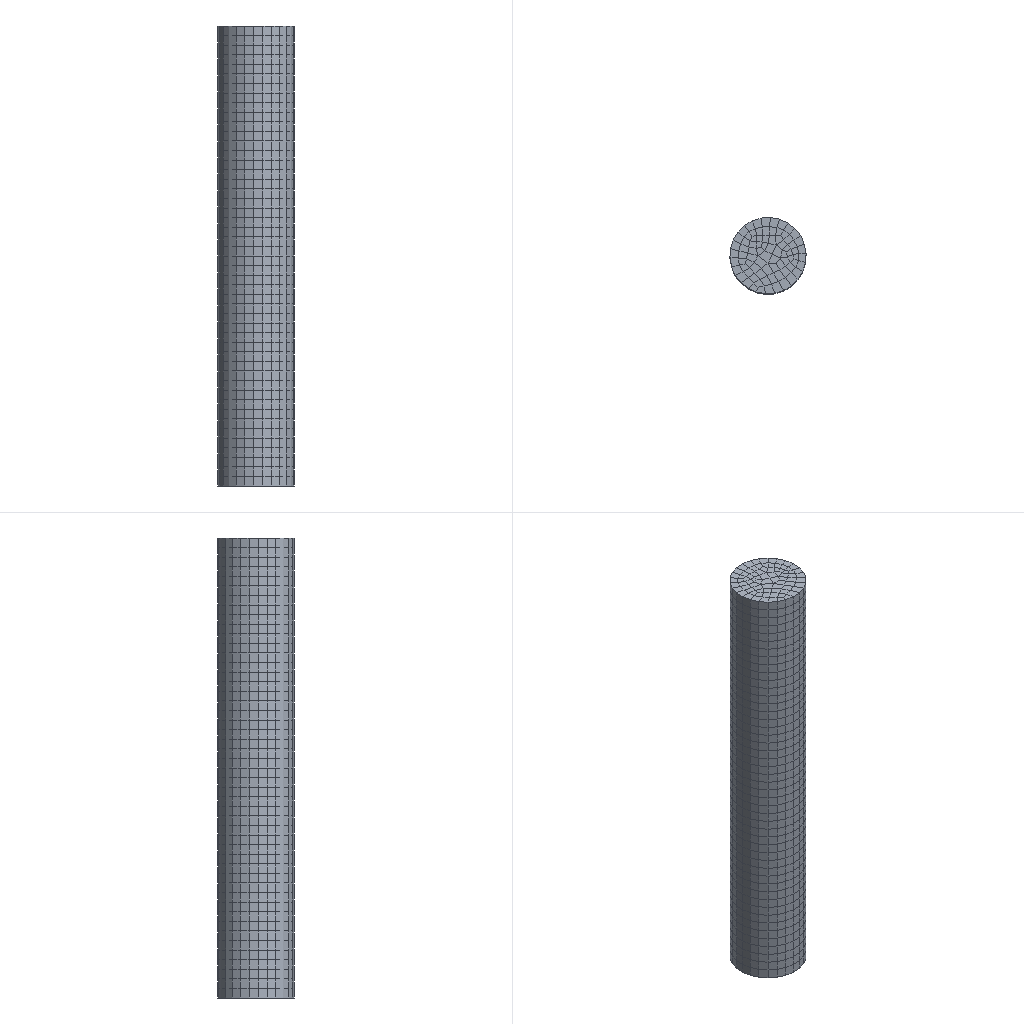Simulation study | abaqus
Set-up summary:
category,name,step,type,value,unit,region
solver,abaqus
solver,version,,,Abaqus/Explicit 2020
units,not stated in the deck,,not stated
analysis,deck,,transient,transient
load_step,Step-1,Step-1,transient
load_step,requested,,,1
mesh,nodes,,,17545
mesh,elements,,,16909
element_type,R3D3,,rigid,125
element_type,R3D4,,rigid,12992
element_type,C3D8R,,solid,3792
load,load commands in deck,,count,1
bc,support commands in deck,,count,7
material,TI,,in results
check,setup vs results,,match,"per instance, exact: element labels, types and connectivity; labels of the nodes the elements use; coordinates of those nodes at SINGLE_PRECISION in 3 of 3 instance(s)"
Abaqus input file, long lists of numbers shortened:
*Heading
** Job name: Job-1 Model name: Model-1
** Generated by: Abaqus/CAE 2020
*Preprint, echo=NO, model=NO, history=NO, contact=NO
**
** PARTS
**
*Part, name=chudun-2
*Node
      1,  -88.649,  -41.876,          90.
      2,  -88.649,  -41.876,         120.
** (8718 more lines like these left out)
*Element, type=R3D4
  1,    1,    7,  341,  388
  2,    7,    8,  342,  341
** (8690 more lines like these left out)
*Element, type=R3D3
6564, 7699, 6751, 7323
6565, 7752, 7314, 7227
** (54 more lines like these left out)
*Node
   8721,  -88.649,  -53.376,         120.
*Nset, nset=chudun-2-RefPt_, internal
8721,
*Elset, elset=chudun-2, generate
    1,  8748,     1
*End Part
**
*Part, name=chudun-4
*Node
      1,  -111.619,  -53.376,          15.
      2,  -111.619,  -53.376,          16.
** (4264 more lines like these left out)
*Element, type=R3D4
  1,   1,   6, 104,   2
  2,   6,   7, 105, 104
** (4298 more lines like these left out)
*Element, type=R3D3
1030, 1237, 1243, 1314
1031, 1266, 1262, 1236
** (67 more lines like these left out)
*Node
   4267,  -88.649,  -53.376,          15.
*Nset, nset=chudun-4-RefPt_, internal
4267,
*Elset, elset=chudun-4, generate
    1,  4369,     1
*End Part
**
*Part, name=xiancai
*Node
      1,   1.19,   3.819,   48.2
      2,  0.2415,   3.993,   48.2
** (4555 more lines like these left out)
*Element, type=C3D8R
   1,  109,   94,  133,  120,   16,    1,   40,   27
   2,  121,   95,  110,  134,   28,    2,   17,   41
** (3790 more lines like these left out)
*Nset, nset=Set-1, generate
    1,  4557,     1
*Elset, elset=Set-1, generate
    1,  3792,     1
** Section: Section-1
*Solid Section, elset=Set-1, material=ti
,
*End Part
**
**
** ASSEMBLY
**
*Assembly, name=Assembly
**
*Instance, name=xiancai-1, part=xiancai
          0.,           0.,        -104.
*End Instance
**
*Instance, name=chudun-2-1, part=chudun-2
   88.649,    53.376,        -120.
*End Instance
**
*Instance, name=chudun-4-1, part=chudun-4
   88.649,    53.376,        -120.
*End Instance
**
*Nset, nset=Set-2, instance=xiancai-1, generate
 4465,  4557,     1
*Elset, elset=Set-2, instance=xiancai-1, generate
 3714,  3792,     1
*Nset, nset=Set-3, instance=chudun-2-1
 8721,
*Nset, nset=Set-3, instance=chudun-4-1
 4267,
*Nset, nset=Set-4, instance=xiancai-1, generate
  1,  93,   1
*Elset, elset=Set-4, instance=xiancai-1, generate
  1,  79,   1
*Rigid Body, ref node=chudun-2-1.chudun-2-RefPt_, elset=chudun-2-1.chudun-2
*Rigid Body, ref node=chudun-4-1.chudun-4-RefPt_, elset=chudun-4-1.chudun-4
*End Assembly
*Amplitude, name=Amp-1
             0.,              0.,             0.1,              1.
**
** MATERIALS
**
*Material, name=ti
*Density
 3.5e-09,
*Elastic
45000., 0.28
*Plastic
300.,0.
**
** INTERACTION PROPERTIES
**
*Surface Interaction, name=IntProp-1
*Friction
 0.01,
*Surface Behavior, pressure-overclosure=HARD
** ----------------------------------------------------------------
**
** STEP: Step-1
**
*Step, name=Step-1, nlgeom=YES
*Dynamic, Explicit
, 0.1
*Bulk Viscosity
0.06, 1.2
** Mass Scaling: Semi-Automatic
**               Whole Model
*Fixed Mass Scaling, factor=5000.
**
** BOUNDARY CONDITIONS
**
** Name: BC-1 Type: 对称/反对称/完全固定
*Boundary
Set-3, ENCASTRE
** Name: BC-2 Type: 位移/转角
*Boundary, amplitude=Amp-1
Set-4, 1, 1
Set-4, 2, 2
Set-4, 3, 3, -25.
Set-4, 4, 4
Set-4, 5, 5
Set-4, 6, 6
**
** INTERACTIONS
**
** Interaction: Int-1
*Contact, op=NEW
*Contact Inclusions, ALL EXTERIOR
*Contact Property Assignment
 ,  , IntProp-1
**
** OUTPUT REQUESTS
**
*Restart, write, number interval=1, time marks=NO
**
** FIELD OUTPUT: F-Output-1
**
*Output, field, number interval=50
*Node Output
A, RF, RM, RT, U, V
*Element Output, directions=YES
E, EVF, LE, MISES, PE, PEEQ, PEEQVAVG, PEVAVG, S, SVAVG
*Contact Output
CDISP, CSTRESS, PPRESS
**
** HISTORY OUTPUT: H-Output-1
**
*Output, history, variable=PRESELECT
*End Step
Results summary:
result,step,Step-1,partial,increments=25233 time=0.08551/0.1
result,analysis,,,transient
result,last_loadstep,,,1
result,primary field,,,U
result,reaction total,,FX,-317.136,model units
result,reaction total,,FY,682.906,model units
result,reaction total,,FZ,361.423,model units